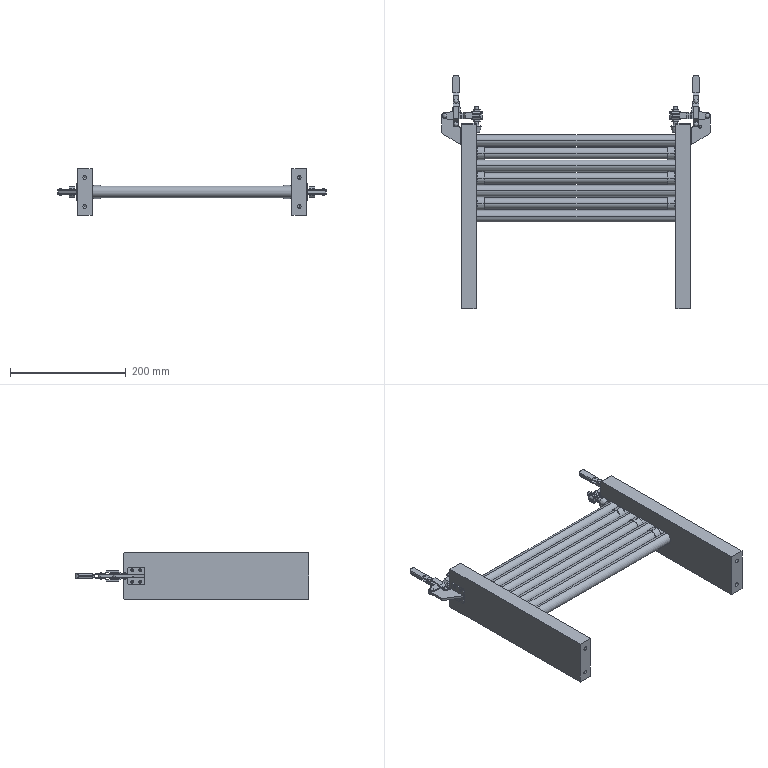Part | SolidWorks | features ReferencePattern 10, LocalLPattern 2, AEMSimFeature 1 | 25 solids | 640 faces | box 463.4 x 403.3 x 80 mm | volume 2031075 mm3 | plane 304 | cylinder 230 | cone 90 | spline 16 | commonest cylinder face diameters 4.8 x48 20 x26 6 x18 3.3 x16 6.8 x16 10 x16